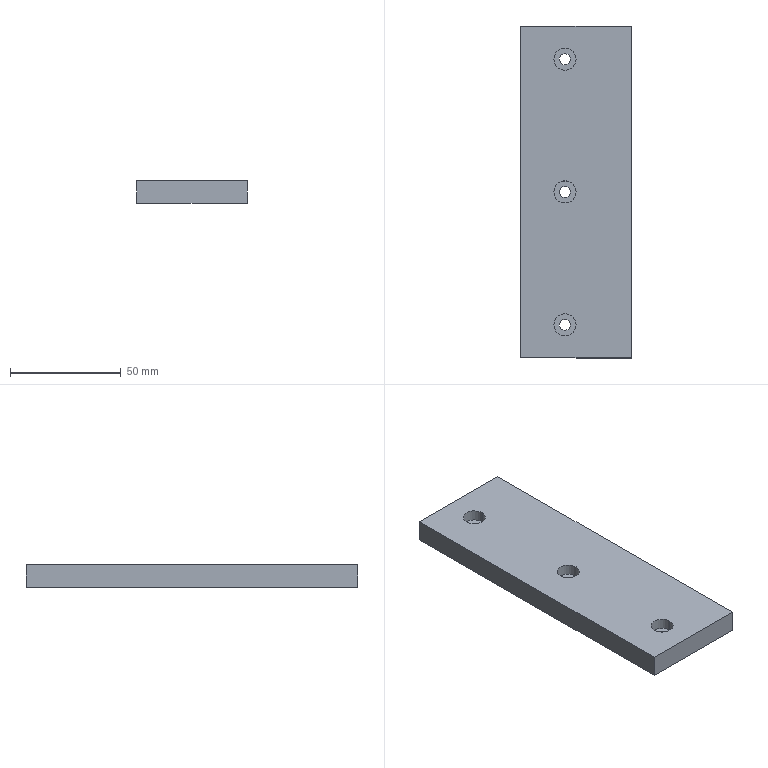Part | SolidWorks | features Chamfer 1, Extrusion 1, HoleWzd 1 | 1 solid | 21 faces | box 50 x 150 x 10 mm | volume 73527 mm3 | cylinder 12 | plane 9 | commonest cylinder face diameters 5 x6 10 x6
STEP:
#1=CARTESIAN_POINT('',(-10.,60.,0.));
#2=VERTEX_POINT('',#1);
#3=CARTESIAN_POINT('',(0.,60.,0.));
#4=VERTEX_POINT('',#3);
#5=CARTESIAN_POINT('',(-5.,60.,0.));
#6=DIRECTION('',(0.,0.,1.));
#7=DIRECTION('',(1.,0.,0.));
#8=AXIS2_PLACEMENT_3D('',#5,#6,#7);
#9=CIRCLE('',#8,5.);
#10=EDGE_CURVE('',#2,#4,#9,.T.);
#11=ORIENTED_EDGE('',*,*,#10,.F.);
#12=CARTESIAN_POINT('',(-10.,60.,5.));
#13=VERTEX_POINT('',#12);
#14=CARTESIAN_POINT('',(-10.,60.,5.));
#15=DIRECTION('',(0.,0.,1.));
#16=VECTOR('',#15,1000.);
#17=LINE('',#14,#16);
#18=EDGE_CURVE('',#2,#13,#17,.T.);
#19=ORIENTED_EDGE('',*,*,#18,.T.);
#20=CARTESIAN_POINT('',(0.,60.,5.));
#21=VERTEX_POINT('',#20);
#22=CARTESIAN_POINT('',(-5.,60.,5.));
#23=DIRECTION('',(0.,0.,1.));
#24=DIRECTION('',(1.,0.,0.));
#25=AXIS2_PLACEMENT_3D('',#22,#23,#24);
#26=CIRCLE('',#25,5.);
#27=EDGE_CURVE('',#13,#21,#26,.T.);
#28=ORIENTED_EDGE('',*,*,#27,.T.);
#29=CARTESIAN_POINT('',(0.,60.,5.));
#30=DIRECTION('',(0.,0.,1.));
#31=VECTOR('',#30,1000.);
#32=LINE('',#29,#31);
#33=EDGE_CURVE('',#4,#21,#32,.T.);
#34=ORIENTED_EDGE('',*,*,#33,.F.);
#35=EDGE_LOOP('',(#11,#19,#28,#34));
#36=FACE_OUTER_BOUND('',#35,.T.);
#37=CARTESIAN_POINT('',(-5.,60.,5.));
#38=DIRECTION('',(0.,0.,1.));
#39=DIRECTION('',(1.,0.,0.));
#40=AXIS2_PLACEMENT_3D('',#37,#38,#39);
#41=CYLINDRICAL_SURFACE('',#40,5.);
#42=ADVANCED_FACE('',(#36),#41,.F.);
#43=CARTESIAN_POINT('',(-7.5,60.,-5.));
#44=VERTEX_POINT('',#43);
#45=CARTESIAN_POINT('',(-2.5,60.,-5.));
#46=VERTEX_POINT('',#45);
#47=CARTESIAN_POINT('',(-5.,60.,-5.));
#48=DIRECTION('',(0.,0.,1.));
#49=DIRECTION('',(1.,0.,0.));
#50=AXIS2_PLACEMENT_3D('',#47,#48,#49);
#51=CIRCLE('',#50,2.5);
#52=EDGE_CURVE('',#44,#46,#51,.T.);
#53=ORIENTED_EDGE('',*,*,#52,.F.);
#54=CARTESIAN_POINT('',(-7.5,60.,0.));
#55=VERTEX_POINT('',#54);
#56=CARTESIAN_POINT('',(-7.5,60.,5.));
#57=DIRECTION('',(0.,0.,1.));
#58=VECTOR('',#57,1000.);
#59=LINE('',#56,#58);
#60=EDGE_CURVE('',#44,#55,#59,.T.);
#61=ORIENTED_EDGE('',*,*,#60,.T.);
#62=CARTESIAN_POINT('',(-2.5,60.,0.));
#63=VERTEX_POINT('',#62);
#64=CARTESIAN_POINT('',(-5.,60.,0.));
#65=DIRECTION('',(0.,0.,1.));
#66=DIRECTION('',(1.,0.,0.));
#67=AXIS2_PLACEMENT_3D('',#64,#65,#66);
#68=CIRCLE('',#67,2.5);
#69=EDGE_CURVE('',#55,#63,#68,.T.);
#70=ORIENTED_EDGE('',*,*,#69,.T.);
#71=CARTESIAN_POINT('',(-2.5,60.,5.));
#72=DIRECTION('',(0.,0.,1.));
#73=VECTOR('',#72,1000.);
#74=LINE('',#71,#73);
#75=EDGE_CURVE('',#46,#63,#74,.T.);
#76=ORIENTED_EDGE('',*,*,#75,.F.);
#77=EDGE_LOOP('',(#53,#61,#70,#76));
#78=FACE_OUTER_BOUND('',#77,.T.);
#79=CARTESIAN_POINT('',(-5.,60.,5.));
#80=DIRECTION('',(0.,0.,1.));
#81=DIRECTION('',(1.,0.,0.));
#82=AXIS2_PLACEMENT_3D('',#79,#80,#81);
#83=CYLINDRICAL_SURFACE('',#82,2.5);
#84=ADVANCED_FACE('',(#78),#83,.F.);
#85=CARTESIAN_POINT('',(-10.,-60.,0.));
#86=VERTEX_POINT('',#85);
#87=CARTESIAN_POINT('',(0.,-60.,0.));
#88=VERTEX_POINT('',#87);
#89=CARTESIAN_POINT('',(-5.,-60.,0.));
#90=DIRECTION('',(0.,0.,1.));
#91=DIRECTION('',(1.,0.,0.));
#92=AXIS2_PLACEMENT_3D('',#89,#90,#91);
#93=CIRCLE('',#92,5.);
#94=EDGE_CURVE('',#86,#88,#93,.T.);
#95=ORIENTED_EDGE('',*,*,#94,.F.);
#96=CARTESIAN_POINT('',(-10.,-60.,5.));
#97=VERTEX_POINT('',#96);
#98=CARTESIAN_POINT('',(-10.,-60.,5.));
#99=DIRECTION('',(0.,0.,1.));
#100=VECTOR('',#99,1000.);
#101=LINE('',#98,#100);
#102=EDGE_CURVE('',#86,#97,#101,.T.);
#103=ORIENTED_EDGE('',*,*,#102,.T.);
#104=CARTESIAN_POINT('',(0.,-60.,5.));
#105=VERTEX_POINT('',#104);
#106=CARTESIAN_POINT('',(-5.,-60.,5.));
#107=DIRECTION('',(0.,0.,1.));
#108=DIRECTION('',(1.,0.,0.));
#109=AXIS2_PLACEMENT_3D('',#106,#107,#108);
#110=CIRCLE('',#109,5.);
#111=EDGE_CURVE('',#97,#105,#110,.T.);
#112=ORIENTED_EDGE('',*,*,#111,.T.);
#113=CARTESIAN_POINT('',(0.,-60.,5.));
#114=DIRECTION('',(0.,0.,1.));
#115=VECTOR('',#114,1000.);
#116=LINE('',#113,#115);
#117=EDGE_CURVE('',#88,#105,#116,.T.);
#118=ORIENTED_EDGE('',*,*,#117,.F.);
#119=EDGE_LOOP('',(#95,#103,#112,#118));
#120=FACE_OUTER_BOUND('',#119,.T.);
#121=CARTESIAN_POINT('',(-5.,-60.,5.));
#122=DIRECTION('',(0.,0.,1.));
#123=DIRECTION('',(1.,0.,0.));
#124=AXIS2_PLACEMENT_3D('',#121,#122,#123);
#125=CYLINDRICAL_SURFACE('',#124,5.);
#126=ADVANCED_FACE('',(#120),#125,.F.);
#127=CARTESIAN_POINT('',(-7.5,-60.,-5.));
#128=VERTEX_POINT('',#127);
#129=CARTESIAN_POINT('',(-2.5,-60.,-5.));
#130=VERTEX_POINT('',#129);
#131=CARTESIAN_POINT('',(-5.,-60.,-5.));
#132=DIRECTION('',(0.,0.,1.));
#133=DIRECTION('',(1.,0.,0.));
#134=AXIS2_PLACEMENT_3D('',#131,#132,#133);
#135=CIRCLE('',#134,2.5);
#136=EDGE_CURVE('',#128,#130,#135,.T.);
#137=ORIENTED_EDGE('',*,*,#136,.F.);
#138=CARTESIAN_POINT('',(-7.5,-60.,0.));
#139=VERTEX_POINT('',#138);
#140=CARTESIAN_POINT('',(-7.5,-60.,5.));
#141=DIRECTION('',(0.,0.,1.));
#142=VECTOR('',#141,1000.);
#143=LINE('',#140,#142);
#144=EDGE_CURVE('',#128,#139,#143,.T.);
#145=ORIENTED_EDGE('',*,*,#144,.T.);
#146=CARTESIAN_POINT('',(-2.5,-60.,0.));
#147=VERTEX_POINT('',#146);
#148=CARTESIAN_POINT('',(-5.,-60.,0.));
#149=DIRECTION('',(0.,0.,1.));
#150=DIRECTION('',(1.,0.,0.));
#151=AXIS2_PLACEMENT_3D('',#148,#149,#150);
#152=CIRCLE('',#151,2.5);
#153=EDGE_CURVE('',#139,#147,#152,.T.);
#154=ORIENTED_EDGE('',*,*,#153,.T.);
#155=CARTESIAN_POINT('',(-2.5,-60.,5.));
#156=DIRECTION('',(0.,0.,1.));
#157=VECTOR('',#156,1000.);
#158=LINE('',#155,#157);
#159=EDGE_CURVE('',#130,#147,#158,.T.);
#160=ORIENTED_EDGE('',*,*,#159,.F.);
#161=EDGE_LOOP('',(#137,#145,#154,#160));
#162=FACE_OUTER_BOUND('',#161,.T.);
#163=CARTESIAN_POINT('',(-5.,-60.,5.));
#164=DIRECTION('',(0.,0.,1.));
#165=DIRECTION('',(1.,0.,0.));
#166=AXIS2_PLACEMENT_3D('',#163,#164,#165);
#167=CYLINDRICAL_SURFACE('',#166,2.5);
#168=ADVANCED_FACE('',(#162),#167,.F.);
#169=CARTESIAN_POINT('',(-10.,0.,0.));
#170=VERTEX_POINT('',#169);
#171=CARTESIAN_POINT('',(0.,0.,0.));
#172=VERTEX_POINT('',#171);
#173=CARTESIAN_POINT('',(-5.,0.,0.));
#174=DIRECTION('',(0.,0.,1.));
#175=DIRECTION('',(1.,0.,0.));
#176=AXIS2_PLACEMENT_3D('',#173,#174,#175);
#177=CIRCLE('',#176,5.);
#178=EDGE_CURVE('',#170,#172,#177,.T.);
#179=ORIENTED_EDGE('',*,*,#178,.F.);
#180=CARTESIAN_POINT('',(-10.,0.,5.));
#181=VERTEX_POINT('',#180);
#182=CARTESIAN_POINT('',(-10.,0.,5.));
#183=DIRECTION('',(0.,0.,1.));
#184=VECTOR('',#183,1000.);
#185=LINE('',#182,#184);
#186=EDGE_CURVE('',#170,#181,#185,.T.);
#187=ORIENTED_EDGE('',*,*,#186,.T.);
#188=CARTESIAN_POINT('',(0.,0.,5.));
#189=VERTEX_POINT('',#188);
#190=CARTESIAN_POINT('',(-5.,0.,5.));
#191=DIRECTION('',(0.,0.,1.));
#192=DIRECTION('',(1.,0.,0.));
#193=AXIS2_PLACEMENT_3D('',#190,#191,#192);
#194=CIRCLE('',#193,5.);
#195=EDGE_CURVE('',#181,#189,#194,.T.);
#196=ORIENTED_EDGE('',*,*,#195,.T.);
#197=CARTESIAN_POINT('',(0.,0.,5.));
#198=DIRECTION('',(0.,0.,1.));
#199=VECTOR('',#198,1000.);
#200=LINE('',#197,#199);
#201=EDGE_CURVE('',#172,#189,#200,.T.);
#202=ORIENTED_EDGE('',*,*,#201,.F.);
#203=EDGE_LOOP('',(#179,#187,#196,#202));
#204=FACE_OUTER_BOUND('',#203,.T.);
#205=CARTESIAN_POINT('',(-5.,0.,5.));
#206=DIRECTION('',(0.,0.,1.));
#207=DIRECTION('',(1.,0.,0.));
#208=AXIS2_PLACEMENT_3D('',#205,#206,#207);
#209=CYLINDRICAL_SURFACE('',#208,5.);
#210=ADVANCED_FACE('',(#204),#209,.F.);
#211=CARTESIAN_POINT('',(-7.5,0.,-5.));
#212=VERTEX_POINT('',#211);
#213=CARTESIAN_POINT('',(-2.5,0.,-5.));
#214=VERTEX_POINT('',#213);
#215=CARTESIAN_POINT('',(-5.,0.,-5.));
#216=DIRECTION('',(0.,0.,1.));
#217=DIRECTION('',(1.,0.,0.));
#218=AXIS2_PLACEMENT_3D('',#215,#216,#217);
#219=CIRCLE('',#218,2.5);
#220=EDGE_CURVE('',#212,#214,#219,.T.);
#221=ORIENTED_EDGE('',*,*,#220,.F.);
#222=CARTESIAN_POINT('',(-7.5,0.,0.));
#223=VERTEX_POINT('',#222);
#224=CARTESIAN_POINT('',(-7.5,0.,5.));
#225=DIRECTION('',(0.,0.,1.));
#226=VECTOR('',#225,1000.);
#227=LINE('',#224,#226);
#228=EDGE_CURVE('',#212,#223,#227,.T.);
#229=ORIENTED_EDGE('',*,*,#228,.T.);
#230=CARTESIAN_POINT('',(-2.5,0.,0.));
#231=VERTEX_POINT('',#230);
#232=CARTESIAN_POINT('',(-5.,0.,0.));
#233=DIRECTION('',(0.,0.,1.));
#234=DIRECTION('',(1.,0.,0.));
#235=AXIS2_PLACEMENT_3D('',#232,#233,#234);
#236=CIRCLE('',#235,2.5);
#237=EDGE_CURVE('',#223,#231,#236,.T.);
#238=ORIENTED_EDGE('',*,*,#237,.T.);
#239=CARTESIAN_POINT('',(-2.5,0.,5.));
#240=DIRECTION('',(0.,0.,1.));
#241=VECTOR('',#240,1000.);
#242=LINE('',#239,#241);
#243=EDGE_CURVE('',#214,#231,#242,.T.);
#244=ORIENTED_EDGE('',*,*,#243,.F.);
#245=EDGE_LOOP('',(#221,#229,#238,#244));
#246=FACE_OUTER_BOUND('',#245,.T.);
#247=CARTESIAN_POINT('',(-5.,0.,5.));
#248=DIRECTION('',(0.,0.,1.));
#249=DIRECTION('',(1.,0.,0.));
#250=AXIS2_PLACEMENT_3D('',#247,#248,#249);
#251=CYLINDRICAL_SURFACE('',#250,2.5);
#252=ADVANCED_FACE('',(#246),#251,.F.);
#253=CARTESIAN_POINT('',(-25.,75.,-5.));
#254=VERTEX_POINT('',#253);
#255=CARTESIAN_POINT('',(-25.,-75.,-5.));
#256=VERTEX_POINT('',#255);
#257=CARTESIAN_POINT('',(-25.,-75.,-5.));
#258=DIRECTION('',(0.,-1.,0.));
#259=VECTOR('',#258,1000.);
#260=LINE('',#257,#259);
#261=EDGE_CURVE('',#254,#256,#260,.T.);
#262=ORIENTED_EDGE('',*,*,#261,.T.);
#263=CARTESIAN_POINT('',(-25.,-75.,5.));
#264=VERTEX_POINT('',#263);
#265=CARTESIAN_POINT('',(-25.,-75.,5.));
#266=DIRECTION('',(0.,0.,-1.));
#267=VECTOR('',#266,1000.);
#268=LINE('',#265,#267);
#269=EDGE_CURVE('',#264,#256,#268,.T.);
#270=ORIENTED_EDGE('',*,*,#269,.F.);
#271=CARTESIAN_POINT('',(-25.,75.,5.));
#272=VERTEX_POINT('',#271);
#273=CARTESIAN_POINT('',(-25.,-75.,5.));
#274=DIRECTION('',(0.,-1.,0.));
#275=VECTOR('',#274,1000.);
#276=LINE('',#273,#275);
#277=EDGE_CURVE('',#272,#264,#276,.T.);
#278=ORIENTED_EDGE('',*,*,#277,.F.);
#279=CARTESIAN_POINT('',(-25.,75.,5.));
#280=DIRECTION('',(0.,0.,-1.));
#281=VECTOR('',#280,1000.);
#282=LINE('',#279,#281);
#283=EDGE_CURVE('',#272,#254,#282,.T.);
#284=ORIENTED_EDGE('',*,*,#283,.T.);
#285=EDGE_LOOP('',(#262,#270,#278,#284));
#286=FACE_OUTER_BOUND('',#285,.T.);
#287=CARTESIAN_POINT('',(-25.,-75.,5.));
#288=DIRECTION('',(1.,0.,0.));
#289=DIRECTION('',(0.,0.,-1.));
#290=AXIS2_PLACEMENT_3D('',#287,#288,#289);
#291=PLANE('',#290);
#292=ADVANCED_FACE('',(#286),#291,.F.);
#293=CARTESIAN_POINT('',(25.,-75.,-5.));
#294=VERTEX_POINT('',#293);
#295=CARTESIAN_POINT('',(25.,-75.,-5.));
#296=DIRECTION('',(1.,0.,0.));
#297=VECTOR('',#296,1000.);
#298=LINE('',#295,#297);
#299=EDGE_CURVE('',#256,#294,#298,.T.);
#300=ORIENTED_EDGE('',*,*,#299,.T.);
#301=CARTESIAN_POINT('',(25.,-75.,5.));
#302=VERTEX_POINT('',#301);
#303=CARTESIAN_POINT('',(25.,-75.,5.));
#304=DIRECTION('',(0.,0.,-1.));
#305=VECTOR('',#304,1000.);
#306=LINE('',#303,#305);
#307=EDGE_CURVE('',#302,#294,#306,.T.);
#308=ORIENTED_EDGE('',*,*,#307,.F.);
#309=CARTESIAN_POINT('',(25.,-75.,5.));
#310=DIRECTION('',(1.,0.,0.));
#311=VECTOR('',#310,1000.);
#312=LINE('',#309,#311);
#313=EDGE_CURVE('',#264,#302,#312,.T.);
#314=ORIENTED_EDGE('',*,*,#313,.F.);
#315=ORIENTED_EDGE('',*,*,#269,.T.);
#316=EDGE_LOOP('',(#300,#308,#314,#315));
#317=FACE_OUTER_BOUND('',#316,.T.);
#318=CARTESIAN_POINT('',(25.,-75.,5.));
#319=DIRECTION('',(0.,1.,0.));
#320=DIRECTION('',(-1.,0.,0.));
#321=AXIS2_PLACEMENT_3D('',#318,#319,#320);
#322=PLANE('',#321);
#323=ADVANCED_FACE('',(#317),#322,.F.);
#324=CARTESIAN_POINT('',(25.,75.,-5.));
#325=VERTEX_POINT('',#324);
#326=CARTESIAN_POINT('',(25.,-75.,-5.));
#327=DIRECTION('',(0.,1.,0.));
#328=VECTOR('',#327,1000.);
#329=LINE('',#326,#328);
#330=EDGE_CURVE('',#294,#325,#329,.T.);
#331=ORIENTED_EDGE('',*,*,#330,.T.);
#332=CARTESIAN_POINT('',(25.,75.,5.));
#333=VERTEX_POINT('',#332);
#334=CARTESIAN_POINT('',(25.,75.,5.));
#335=DIRECTION('',(0.,0.,-1.));
#336=VECTOR('',#335,1000.);
#337=LINE('',#334,#336);
#338=EDGE_CURVE('',#333,#325,#337,.T.);
#339=ORIENTED_EDGE('',*,*,#338,.F.);
#340=CARTESIAN_POINT('',(25.,-75.,5.));
#341=DIRECTION('',(0.,1.,0.));
#342=VECTOR('',#341,1000.);
#343=LINE('',#340,#342);
#344=EDGE_CURVE('',#302,#333,#343,.T.);
#345=ORIENTED_EDGE('',*,*,#344,.F.);
#346=ORIENTED_EDGE('',*,*,#307,.T.);
#347=EDGE_LOOP('',(#331,#339,#345,#346));
#348=FACE_OUTER_BOUND('',#347,.T.);
#349=CARTESIAN_POINT('',(25.,-75.,5.));
#350=DIRECTION('',(-1.,0.,0.));
#351=DIRECTION('',(0.,0.,1.));
#352=AXIS2_PLACEMENT_3D('',#349,#350,#351);
#353=PLANE('',#352);
#354=ADVANCED_FACE('',(#348),#353,.F.);
#355=CARTESIAN_POINT('',(25.,75.,-5.));
#356=DIRECTION('',(-1.,0.,0.));
#357=VECTOR('',#356,1000.);
#358=LINE('',#355,#357);
#359=EDGE_CURVE('',#325,#254,#358,.T.);
#360=ORIENTED_EDGE('',*,*,#359,.T.);
#361=ORIENTED_EDGE('',*,*,#283,.F.);
#362=CARTESIAN_POINT('',(25.,75.,5.));
#363=DIRECTION('',(-1.,0.,0.));
#364=VECTOR('',#363,1000.);
#365=LINE('',#362,#364);
#366=EDGE_CURVE('',#333,#272,#365,.T.);
#367=ORIENTED_EDGE('',*,*,#366,.F.);
#368=ORIENTED_EDGE('',*,*,#338,.T.);
#369=EDGE_LOOP('',(#360,#361,#367,#368));
#370=FACE_OUTER_BOUND('',#369,.T.);
#371=CARTESIAN_POINT('',(25.,75.,5.));
#372=DIRECTION('',(0.,-1.,0.));
#373=DIRECTION('',(0.,0.,-1.));
#374=AXIS2_PLACEMENT_3D('',#371,#372,#373);
#375=PLANE('',#374);
#376=ADVANCED_FACE('',(#370),#375,.F.);
#377=CARTESIAN_POINT('',(-5.,60.,5.));
#378=DIRECTION('',(0.,0.,1.));
#379=DIRECTION('',(1.,0.,0.));
#380=AXIS2_PLACEMENT_3D('',#377,#378,#379);
#381=CIRCLE('',#380,5.);
#382=EDGE_CURVE('',#21,#13,#381,.T.);
#383=ORIENTED_EDGE('',*,*,#382,.F.);
#384=ORIENTED_EDGE('',*,*,#27,.F.);
#385=EDGE_LOOP('',(#383,#384));
#386=FACE_BOUND('',#385,.T.);
#387=CARTESIAN_POINT('',(-5.,-60.,5.));
#388=DIRECTION('',(0.,0.,1.));
#389=DIRECTION('',(1.,0.,0.));
#390=AXIS2_PLACEMENT_3D('',#387,#388,#389);
#391=CIRCLE('',#390,5.);
#392=EDGE_CURVE('',#105,#97,#391,.T.);
#393=ORIENTED_EDGE('',*,*,#392,.F.);
#394=ORIENTED_EDGE('',*,*,#111,.F.);
#395=EDGE_LOOP('',(#393,#394));
#396=FACE_BOUND('',#395,.T.);
#397=CARTESIAN_POINT('',(-5.,0.,5.));
#398=DIRECTION('',(0.,0.,1.));
#399=DIRECTION('',(1.,0.,0.));
#400=AXIS2_PLACEMENT_3D('',#397,#398,#399);
#401=CIRCLE('',#400,5.);
#402=EDGE_CURVE('',#189,#181,#401,.T.);
#403=ORIENTED_EDGE('',*,*,#402,.F.);
#404=ORIENTED_EDGE('',*,*,#195,.F.);
#405=EDGE_LOOP('',(#403,#404));
#406=FACE_BOUND('',#405,.T.);
#407=ORIENTED_EDGE('',*,*,#277,.T.);
#408=ORIENTED_EDGE('',*,*,#313,.T.);
#409=ORIENTED_EDGE('',*,*,#344,.T.);
#410=ORIENTED_EDGE('',*,*,#366,.T.);
#411=EDGE_LOOP('',(#407,#408,#409,#410));
#412=FACE_OUTER_BOUND('',#411,.T.);
#413=CARTESIAN_POINT('',(0.,0.,5.));
#414=DIRECTION('',(0.,0.,1.));
#415=DIRECTION('',(1.,0.,0.));
#416=AXIS2_PLACEMENT_3D('',#413,#414,#415);
#417=PLANE('',#416);
#418=ADVANCED_FACE('',(#386,#396,#406,#412),#417,.T.);
#419=CARTESIAN_POINT('',(-5.,60.,-5.));
#420=DIRECTION('',(0.,0.,1.));
#421=DIRECTION('',(1.,0.,0.));
#422=AXIS2_PLACEMENT_3D('',#419,#420,#421);
#423=CIRCLE('',#422,2.5);
#424=EDGE_CURVE('',#46,#44,#423,.T.);
#425=ORIENTED_EDGE('',*,*,#424,.T.);
#426=ORIENTED_EDGE('',*,*,#52,.T.);
#427=EDGE_LOOP('',(#425,#426));
#428=FACE_BOUND('',#427,.T.);
#429=CARTESIAN_POINT('',(-5.,-60.,-5.));
#430=DIRECTION('',(0.,0.,1.));
#431=DIRECTION('',(1.,0.,0.));
#432=AXIS2_PLACEMENT_3D('',#429,#430,#431);
#433=CIRCLE('',#432,2.5);
#434=EDGE_CURVE('',#130,#128,#433,.T.);
#435=ORIENTED_EDGE('',*,*,#434,.T.);
#436=ORIENTED_EDGE('',*,*,#136,.T.);
#437=EDGE_LOOP('',(#435,#436));
#438=FACE_BOUND('',#437,.T.);
#439=CARTESIAN_POINT('',(-5.,0.,-5.));
#440=DIRECTION('',(0.,0.,1.));
#441=DIRECTION('',(1.,0.,0.));
#442=AXIS2_PLACEMENT_3D('',#439,#440,#441);
#443=CIRCLE('',#442,2.5);
#444=EDGE_CURVE('',#214,#212,#443,.T.);
#445=ORIENTED_EDGE('',*,*,#444,.T.);
#446=ORIENTED_EDGE('',*,*,#220,.T.);
#447=EDGE_LOOP('',(#445,#446));
#448=FACE_BOUND('',#447,.T.);
#449=ORIENTED_EDGE('',*,*,#261,.F.);
#450=ORIENTED_EDGE('',*,*,#359,.F.);
#451=ORIENTED_EDGE('',*,*,#330,.F.);
#452=ORIENTED_EDGE('',*,*,#299,.F.);
#453=EDGE_LOOP('',(#449,#450,#451,#452));
#454=FACE_OUTER_BOUND('',#453,.T.);
#455=CARTESIAN_POINT('',(0.,0.,-5.));
#456=DIRECTION('',(0.,0.,1.));
#457=DIRECTION('',(1.,0.,0.));
#458=AXIS2_PLACEMENT_3D('',#455,#456,#457);
#459=PLANE('',#458);
#460=ADVANCED_FACE('',(#428,#438,#448,#454),#459,.F.);
#461=ORIENTED_EDGE('',*,*,#228,.F.);
#462=ORIENTED_EDGE('',*,*,#444,.F.);
#463=ORIENTED_EDGE('',*,*,#243,.T.);
#464=CARTESIAN_POINT('',(-5.,0.,0.));
#465=DIRECTION('',(0.,0.,1.));
#466=DIRECTION('',(1.,0.,0.));
#467=AXIS2_PLACEMENT_3D('',#464,#465,#466);
#468=CIRCLE('',#467,2.5);
#469=EDGE_CURVE('',#231,#223,#468,.T.);
#470=ORIENTED_EDGE('',*,*,#469,.T.);
#471=EDGE_LOOP('',(#461,#462,#463,#470));
#472=FACE_OUTER_BOUND('',#471,.T.);
#473=CARTESIAN_POINT('',(-5.,0.,5.));
#474=DIRECTION('',(0.,0.,1.));
#475=DIRECTION('',(1.,0.,0.));
#476=AXIS2_PLACEMENT_3D('',#473,#474,#475);
#477=CYLINDRICAL_SURFACE('',#476,2.5);
#478=ADVANCED_FACE('',(#472),#477,.F.);
#479=ORIENTED_EDGE('',*,*,#469,.F.);
#480=ORIENTED_EDGE('',*,*,#237,.F.);
#481=EDGE_LOOP('',(#479,#480));
#482=FACE_BOUND('',#481,.T.);
#483=CARTESIAN_POINT('',(-5.,0.,0.));
#484=DIRECTION('',(0.,0.,1.));
#485=DIRECTION('',(1.,0.,0.));
#486=AXIS2_PLACEMENT_3D('',#483,#484,#485);
#487=CIRCLE('',#486,5.);
#488=EDGE_CURVE('',#172,#170,#487,.T.);
#489=ORIENTED_EDGE('',*,*,#488,.T.);
#490=ORIENTED_EDGE('',*,*,#178,.T.);
#491=EDGE_LOOP('',(#489,#490));
#492=FACE_OUTER_BOUND('',#491,.T.);
#493=CARTESIAN_POINT('',(-2.5,0.,0.));
#494=DIRECTION('',(0.,0.,-1.));
#495=DIRECTION('',(-1.,0.,0.));
#496=AXIS2_PLACEMENT_3D('',#493,#494,#495);
#497=PLANE('',#496);
#498=ADVANCED_FACE('',(#482,#492),#497,.F.);
#499=ORIENTED_EDGE('',*,*,#186,.F.);
#500=ORIENTED_EDGE('',*,*,#488,.F.);
#501=ORIENTED_EDGE('',*,*,#201,.T.);
#502=ORIENTED_EDGE('',*,*,#402,.T.);
#503=EDGE_LOOP('',(#499,#500,#501,#502));
#504=FACE_OUTER_BOUND('',#503,.T.);
#505=CARTESIAN_POINT('',(-5.,0.,5.));
#506=DIRECTION('',(0.,0.,1.));
#507=DIRECTION('',(1.,0.,0.));
#508=AXIS2_PLACEMENT_3D('',#505,#506,#507);
#509=CYLINDRICAL_SURFACE('',#508,5.);
#510=ADVANCED_FACE('',(#504),#509,.F.);
#511=ORIENTED_EDGE('',*,*,#144,.F.);
#512=ORIENTED_EDGE('',*,*,#434,.F.);
#513=ORIENTED_EDGE('',*,*,#159,.T.);
#514=CARTESIAN_POINT('',(-5.,-60.,0.));
#515=DIRECTION('',(0.,0.,1.));
#516=DIRECTION('',(1.,0.,0.));
#517=AXIS2_PLACEMENT_3D('',#514,#515,#516);
#518=CIRCLE('',#517,2.5);
#519=EDGE_CURVE('',#147,#139,#518,.T.);
#520=ORIENTED_EDGE('',*,*,#519,.T.);
#521=EDGE_LOOP('',(#511,#512,#513,#520));
#522=FACE_OUTER_BOUND('',#521,.T.);
#523=CARTESIAN_POINT('',(-5.,-60.,5.));
#524=DIRECTION('',(0.,0.,1.));
#525=DIRECTION('',(1.,0.,0.));
#526=AXIS2_PLACEMENT_3D('',#523,#524,#525);
#527=CYLINDRICAL_SURFACE('',#526,2.5);
#528=ADVANCED_FACE('',(#522),#527,.F.);
#529=ORIENTED_EDGE('',*,*,#519,.F.);
#530=ORIENTED_EDGE('',*,*,#153,.F.);
#531=EDGE_LOOP('',(#529,#530));
#532=FACE_BOUND('',#531,.T.);
#533=CARTESIAN_POINT('',(-5.,-60.,0.));
#534=DIRECTION('',(0.,0.,1.));
#535=DIRECTION('',(1.,0.,0.));
#536=AXIS2_PLACEMENT_3D('',#533,#534,#535);
#537=CIRCLE('',#536,5.);
#538=EDGE_CURVE('',#88,#86,#537,.T.);
#539=ORIENTED_EDGE('',*,*,#538,.T.);
#540=ORIENTED_EDGE('',*,*,#94,.T.);
#541=EDGE_LOOP('',(#539,#540));
#542=FACE_OUTER_BOUND('',#541,.T.);
#543=CARTESIAN_POINT('',(-2.5,-60.,0.));
#544=DIRECTION('',(0.,0.,-1.));
#545=DIRECTION('',(-1.,0.,0.));
#546=AXIS2_PLACEMENT_3D('',#543,#544,#545);
#547=PLANE('',#546);
#548=ADVANCED_FACE('',(#532,#542),#547,.F.);
#549=ORIENTED_EDGE('',*,*,#102,.F.);
#550=ORIENTED_EDGE('',*,*,#538,.F.);
#551=ORIENTED_EDGE('',*,*,#117,.T.);
#552=ORIENTED_EDGE('',*,*,#392,.T.);
#553=EDGE_LOOP('',(#549,#550,#551,#552));
#554=FACE_OUTER_BOUND('',#553,.T.);
#555=CARTESIAN_POINT('',(-5.,-60.,5.));
#556=DIRECTION('',(0.,0.,1.));
#557=DIRECTION('',(1.,0.,0.));
#558=AXIS2_PLACEMENT_3D('',#555,#556,#557);
#559=CYLINDRICAL_SURFACE('',#558,5.);
#560=ADVANCED_FACE('',(#554),#559,.F.);
#561=ORIENTED_EDGE('',*,*,#60,.F.);
#562=ORIENTED_EDGE('',*,*,#424,.F.);
#563=ORIENTED_EDGE('',*,*,#75,.T.);
#564=CARTESIAN_POINT('',(-5.,60.,0.));
#565=DIRECTION('',(0.,0.,1.));
#566=DIRECTION('',(1.,0.,0.));
#567=AXIS2_PLACEMENT_3D('',#564,#565,#566);
#568=CIRCLE('',#567,2.5);
#569=EDGE_CURVE('',#63,#55,#568,.T.);
#570=ORIENTED_EDGE('',*,*,#569,.T.);
#571=EDGE_LOOP('',(#561,#562,#563,#570));
#572=FACE_OUTER_BOUND('',#571,.T.);
#573=CARTESIAN_POINT('',(-5.,60.,5.));
#574=DIRECTION('',(0.,0.,1.));
#575=DIRECTION('',(1.,0.,0.));
#576=AXIS2_PLACEMENT_3D('',#573,#574,#575);
#577=CYLINDRICAL_SURFACE('',#576,2.5);
#578=ADVANCED_FACE('',(#572),#577,.F.);
#579=ORIENTED_EDGE('',*,*,#569,.F.);
#580=ORIENTED_EDGE('',*,*,#69,.F.);
#581=EDGE_LOOP('',(#579,#580));
#582=FACE_BOUND('',#581,.T.);
#583=CARTESIAN_POINT('',(-5.,60.,0.));
#584=DIRECTION('',(0.,0.,1.));
#585=DIRECTION('',(1.,0.,0.));
#586=AXIS2_PLACEMENT_3D('',#583,#584,#585);
#587=CIRCLE('',#586,5.);
#588=EDGE_CURVE('',#4,#2,#587,.T.);
#589=ORIENTED_EDGE('',*,*,#588,.T.);
#590=ORIENTED_EDGE('',*,*,#10,.T.);
#591=EDGE_LOOP('',(#589,#590));
#592=FACE_OUTER_BOUND('',#591,.T.);
#593=CARTESIAN_POINT('',(-2.5,60.,0.));
#594=DIRECTION('',(0.,0.,-1.));
#595=DIRECTION('',(-1.,0.,0.));
#596=AXIS2_PLACEMENT_3D('',#593,#594,#595);
#597=PLANE('',#596);
#598=ADVANCED_FACE('',(#582,#592),#597,.F.);
#599=ORIENTED_EDGE('',*,*,#18,.F.);
#600=ORIENTED_EDGE('',*,*,#588,.F.);
#601=ORIENTED_EDGE('',*,*,#33,.T.);
#602=ORIENTED_EDGE('',*,*,#382,.T.);
#603=EDGE_LOOP('',(#599,#600,#601,#602));
#604=FACE_OUTER_BOUND('',#603,.T.);
#605=CARTESIAN_POINT('',(-5.,60.,5.));
#606=DIRECTION('',(0.,0.,1.));
#607=DIRECTION('',(1.,0.,0.));
#608=AXIS2_PLACEMENT_3D('',#605,#606,#607);
#609=CYLINDRICAL_SURFACE('',#608,5.);
#610=ADVANCED_FACE('',(#604),#609,.F.);
#611=CLOSED_SHELL('',(#42,#84,#126,#168,#210,#252,#292,#323,#354,#376,#418,#460,#478,#498,#510,#528,#548,#560,#578,#598,#610));
#612=MANIFOLD_SOLID_BREP('',#611);
#613=CARTESIAN_POINT('',(0.,0.,0.));
#614=DIRECTION('',(0.,0.,1.));
#615=DIRECTION('',(1.,0.,0.));
#616=AXIS2_PLACEMENT_3D('',#613,#614,#615);
#617=(LENGTH_UNIT()NAMED_UNIT(*)SI_UNIT(.MILLI.,.METRE.));
#618=UNCERTAINTY_MEASURE_WITH_UNIT(LENGTH_MEASURE(0.00001),#617,'','');
#619=(NAMED_UNIT(*)PLANE_ANGLE_UNIT()SI_UNIT($,.RADIAN.));
#620=(NAMED_UNIT(*)SI_UNIT($,.STERADIAN.)SOLID_ANGLE_UNIT());
#621=(GEOMETRIC_REPRESENTATION_CONTEXT(3)GLOBAL_UNCERTAINTY_ASSIGNED_CONTEXT((#618))GLOBAL_UNIT_ASSIGNED_CONTEXT((#617,#619,#620))REPRESENTATION_CONTEXT('',''));
#622=ADVANCED_BREP_SHAPE_REPRESENTATION('',(#612,#616),#621);